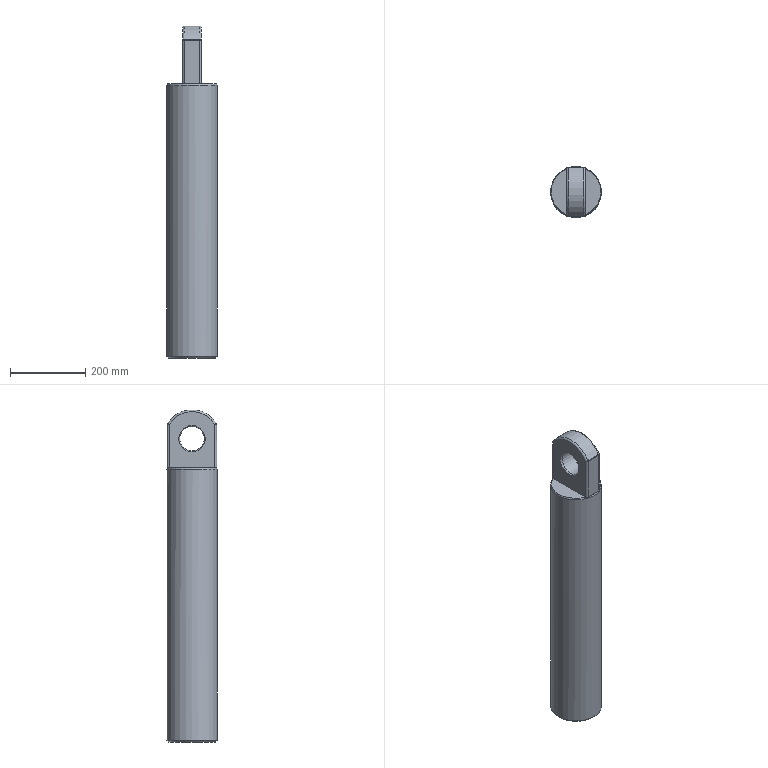Part | NX | features 平衡千斤顶活塞 2 | 1 solid | 32 faces | box 135 x 135 x 882.27 mm | volume 11180627 mm3 | plane 13 | cylinder 9 | cone 4 | sphere 4 | torus 2 | commonest cylinder face diameters 10 x6 65 x1 135 x1 153.5 x1
STEP:
#1=CARTESIAN_POINT('',(-24.997,60.688,727.9));
#2=VERTEX_POINT('',#1);
#3=CARTESIAN_POINT('',(-24.997,-60.688,727.9));
#4=VERTEX_POINT('',#3);
#5=CARTESIAN_POINT('',(0.,0.,727.9));
#6=DIRECTION('',(0.,0.,1.));
#7=DIRECTION('',(1.,0.,0.));
#8=AXIS2_PLACEMENT_3D('',#5,#6,#7);
#9=CIRCLE('',#8,65.635);
#10=EDGE_CURVE('',#2,#4,#9,.T.);
#11=ORIENTED_EDGE('',*,*,#10,.T.);
#12=CARTESIAN_POINT('',(-25.,-60.524,727.9));
#13=VERTEX_POINT('',#12);
#14=CARTESIAN_POINT('',(-20.,-60.524,727.9));
#15=DIRECTION('',(0.,0.,1.));
#16=DIRECTION('',(1.,0.,0.));
#17=AXIS2_PLACEMENT_3D('',#14,#15,#16);
#18=CIRCLE('',#17,5.);
#19=EDGE_CURVE('',#4,#13,#18,.F.);
#20=ORIENTED_EDGE('',*,*,#19,.T.);
#21=CARTESIAN_POINT('',(-25.,60.524,727.9));
#22=VERTEX_POINT('',#21);
#23=CARTESIAN_POINT('',(-25.,65.524,727.9));
#24=DIRECTION('',(0.,1.,0.));
#25=VECTOR('',#24,1000.);
#26=LINE('',#23,#25);
#27=EDGE_CURVE('',#13,#22,#26,.T.);
#28=ORIENTED_EDGE('',*,*,#27,.T.);
#29=CARTESIAN_POINT('',(-20.,60.524,727.9));
#30=DIRECTION('',(0.,0.,1.));
#31=DIRECTION('',(1.,0.,0.));
#32=AXIS2_PLACEMENT_3D('',#29,#30,#31);
#33=CIRCLE('',#32,5.);
#34=EDGE_CURVE('',#22,#2,#33,.F.);
#35=ORIENTED_EDGE('',*,*,#34,.T.);
#36=EDGE_LOOP('',(#11,#20,#28,#35));
#37=FACE_BOUND('',#36,.T.);
#38=CARTESIAN_POINT('',(0.,0.,727.9));
#39=DIRECTION('',(0.,0.,1.));
#40=DIRECTION('',(1.,0.,0.));
#41=AXIS2_PLACEMENT_3D('',#38,#39,#40);
#42=PLANE('',#41);
#43=ADVANCED_FACE('',(#37),#42,.T.);
#44=CARTESIAN_POINT('',(3.807,65.524,727.9));
#45=VERTEX_POINT('',#44);
#46=CARTESIAN_POINT('',(-3.807,65.524,727.9));
#47=VERTEX_POINT('',#46);
#48=CARTESIAN_POINT('',(25.,65.524,727.9));
#49=DIRECTION('',(-1.,0.,0.));
#50=VECTOR('',#49,1000.);
#51=LINE('',#48,#50);
#52=EDGE_CURVE('',#45,#47,#51,.T.);
#53=ORIENTED_EDGE('',*,*,#52,.F.);
#54=CARTESIAN_POINT('',(0.,0.,727.9));
#55=DIRECTION('',(0.,0.,1.));
#56=DIRECTION('',(1.,0.,0.));
#57=AXIS2_PLACEMENT_3D('',#54,#55,#56);
#58=CIRCLE('',#57,65.635);
#59=EDGE_CURVE('',#45,#47,#58,.T.);
#60=ORIENTED_EDGE('',*,*,#59,.T.);
#61=EDGE_LOOP('',(#53,#60));
#62=FACE_BOUND('',#61,.T.);
#63=CARTESIAN_POINT('',(0.,0.,727.9));
#64=DIRECTION('',(0.,0.,1.));
#65=DIRECTION('',(1.,0.,0.));
#66=AXIS2_PLACEMENT_3D('',#63,#64,#65);
#67=PLANE('',#66);
#68=ADVANCED_FACE('',(#62),#67,.T.);
#69=CARTESIAN_POINT('',(-3.816,-65.524,727.9));
#70=VERTEX_POINT('',#69);
#71=CARTESIAN_POINT('',(3.816,-65.524,727.9));
#72=VERTEX_POINT('',#71);
#73=CARTESIAN_POINT('',(0.,0.,727.9));
#74=DIRECTION('',(0.,0.,1.));
#75=DIRECTION('',(1.,0.,0.));
#76=AXIS2_PLACEMENT_3D('',#73,#74,#75);
#77=CIRCLE('',#76,65.635);
#78=EDGE_CURVE('',#70,#72,#77,.T.);
#79=ORIENTED_EDGE('',*,*,#78,.T.);
#80=CARTESIAN_POINT('',(25.,-65.524,727.9));
#81=DIRECTION('',(-1.,0.,0.));
#82=VECTOR('',#81,1000.);
#83=LINE('',#80,#82);
#84=EDGE_CURVE('',#72,#70,#83,.T.);
#85=ORIENTED_EDGE('',*,*,#84,.T.);
#86=EDGE_LOOP('',(#79,#85));
#87=FACE_BOUND('',#86,.T.);
#88=CARTESIAN_POINT('',(0.,0.,727.9));
#89=DIRECTION('',(0.,0.,1.));
#90=DIRECTION('',(1.,0.,0.));
#91=AXIS2_PLACEMENT_3D('',#88,#89,#90);
#92=PLANE('',#91);
#93=ADVANCED_FACE('',(#87),#92,.T.);
#94=CARTESIAN_POINT('',(67.5,0.,723.9));
#95=VERTEX_POINT('',#94);
#96=CARTESIAN_POINT('',(0.,0.,723.9));
#97=DIRECTION('',(0.,0.,1.));
#98=DIRECTION('',(1.,0.,0.));
#99=AXIS2_PLACEMENT_3D('',#96,#97,#98);
#100=CIRCLE('',#99,67.5);
#101=EDGE_CURVE('',#95,#95,#100,.F.);
#102=ORIENTED_EDGE('',*,*,#101,.T.);
#103=EDGE_LOOP('',(#102));
#104=FACE_BOUND('',#103,.T.);
#105=CARTESIAN_POINT('',(67.5,0.,5.));
#106=VERTEX_POINT('',#105);
#107=CARTESIAN_POINT('',(0.,0.,5.));
#108=DIRECTION('',(0.,0.,1.));
#109=DIRECTION('',(1.,0.,0.));
#110=AXIS2_PLACEMENT_3D('',#107,#108,#109);
#111=CIRCLE('',#110,67.5);
#112=EDGE_CURVE('',#106,#106,#111,.T.);
#113=ORIENTED_EDGE('',*,*,#112,.T.);
#114=EDGE_LOOP('',(#113));
#115=FACE_BOUND('',#114,.T.);
#116=CARTESIAN_POINT('',(0.,0.,727.9));
#117=DIRECTION('',(0.,0.,-1.));
#118=DIRECTION('',(-1.,0.,0.));
#119=AXIS2_PLACEMENT_3D('',#116,#117,#118);
#120=CYLINDRICAL_SURFACE('',#119,67.5);
#121=ADVANCED_FACE('',(#104,#115),#120,.T.);
#122=CARTESIAN_POINT('',(25.,-60.524,727.9));
#123=VERTEX_POINT('',#122);
#124=CARTESIAN_POINT('',(25.,60.524,727.9));
#125=VERTEX_POINT('',#124);
#126=CARTESIAN_POINT('',(25.,65.524,727.9));
#127=DIRECTION('',(0.,1.,0.));
#128=VECTOR('',#127,1000.);
#129=LINE('',#126,#128);
#130=EDGE_CURVE('',#123,#125,#129,.T.);
#131=ORIENTED_EDGE('',*,*,#130,.F.);
#132=CARTESIAN_POINT('',(24.997,-60.688,727.9));
#133=VERTEX_POINT('',#132);
#134=CARTESIAN_POINT('',(20.,-60.524,727.9));
#135=DIRECTION('',(0.,0.,1.));
#136=DIRECTION('',(1.,0.,0.));
#137=AXIS2_PLACEMENT_3D('',#134,#135,#136);
#138=CIRCLE('',#137,5.);
#139=EDGE_CURVE('',#123,#133,#138,.F.);
#140=ORIENTED_EDGE('',*,*,#139,.T.);
#141=CARTESIAN_POINT('',(24.997,60.688,727.9));
#142=VERTEX_POINT('',#141);
#143=CARTESIAN_POINT('',(0.,0.,727.9));
#144=DIRECTION('',(0.,0.,1.));
#145=DIRECTION('',(1.,0.,0.));
#146=AXIS2_PLACEMENT_3D('',#143,#144,#145);
#147=CIRCLE('',#146,65.635);
#148=EDGE_CURVE('',#133,#142,#147,.T.);
#149=ORIENTED_EDGE('',*,*,#148,.T.);
#150=CARTESIAN_POINT('',(20.,60.524,727.9));
#151=DIRECTION('',(0.,0.,1.));
#152=DIRECTION('',(1.,0.,0.));
#153=AXIS2_PLACEMENT_3D('',#150,#151,#152);
#154=CIRCLE('',#153,5.);
#155=EDGE_CURVE('',#142,#125,#154,.F.);
#156=ORIENTED_EDGE('',*,*,#155,.T.);
#157=EDGE_LOOP('',(#131,#140,#149,#156));
#158=FACE_BOUND('',#157,.T.);
#159=CARTESIAN_POINT('',(0.,0.,727.9));
#160=DIRECTION('',(0.,0.,1.));
#161=DIRECTION('',(1.,0.,0.));
#162=AXIS2_PLACEMENT_3D('',#159,#160,#161);
#163=PLANE('',#162);
#164=ADVANCED_FACE('',(#158),#163,.T.);
#165=CARTESIAN_POINT('',(62.5,0.,0.));
#166=VERTEX_POINT('',#165);
#167=CARTESIAN_POINT('',(0.,0.,0.));
#168=DIRECTION('',(0.,0.,1.));
#169=DIRECTION('',(1.,0.,0.));
#170=AXIS2_PLACEMENT_3D('',#167,#168,#169);
#171=CIRCLE('',#170,62.5);
#172=EDGE_CURVE('',#166,#166,#171,.F.);
#173=ORIENTED_EDGE('',*,*,#172,.T.);
#174=EDGE_LOOP('',(#173));
#175=FACE_BOUND('',#174,.T.);
#176=CARTESIAN_POINT('',(0.,0.,0.));
#177=DIRECTION('',(0.,0.,1.));
#178=DIRECTION('',(1.,0.,0.));
#179=AXIS2_PLACEMENT_3D('',#176,#177,#178);
#180=PLANE('',#179);
#181=ADVANCED_FACE('',(#175),#180,.F.);
#182=ORIENTED_EDGE('',*,*,#172,.F.);
#183=EDGE_LOOP('',(#182));
#184=FACE_BOUND('',#183,.T.);
#185=ORIENTED_EDGE('',*,*,#112,.F.);
#186=EDGE_LOOP('',(#185));
#187=FACE_BOUND('',#186,.T.);
#188=CARTESIAN_POINT('',(0.,0.,5.));
#189=DIRECTION('',(0.,0.,1.));
#190=DIRECTION('',(1.,0.,0.));
#191=AXIS2_PLACEMENT_3D('',#188,#189,#190);
#192=CONICAL_SURFACE('',#191,67.5,0.7854);
#193=ADVANCED_FACE('',(#184,#187),#192,.T.);
#194=ORIENTED_EDGE('',*,*,#101,.F.);
#195=EDGE_LOOP('',(#194));
#196=FACE_BOUND('',#195,.T.);
#197=CARTESIAN_POINT('',(0.,0.,727.9));
#198=DIRECTION('',(0.,0.,1.));
#199=DIRECTION('',(1.,0.,0.));
#200=AXIS2_PLACEMENT_3D('',#197,#198,#199);
#201=CIRCLE('',#200,65.635);
#202=EDGE_CURVE('',#142,#45,#201,.T.);
#203=ORIENTED_EDGE('',*,*,#202,.F.);
#204=ORIENTED_EDGE('',*,*,#148,.F.);
#205=CARTESIAN_POINT('',(0.,0.,727.9));
#206=DIRECTION('',(0.,0.,1.));
#207=DIRECTION('',(1.,0.,0.));
#208=AXIS2_PLACEMENT_3D('',#205,#206,#207);
#209=CIRCLE('',#208,65.635);
#210=EDGE_CURVE('',#72,#133,#209,.T.);
#211=ORIENTED_EDGE('',*,*,#210,.F.);
#212=ORIENTED_EDGE('',*,*,#78,.F.);
#213=CARTESIAN_POINT('',(0.,0.,727.9));
#214=DIRECTION('',(0.,0.,1.));
#215=DIRECTION('',(1.,0.,0.));
#216=AXIS2_PLACEMENT_3D('',#213,#214,#215);
#217=CIRCLE('',#216,65.635);
#218=EDGE_CURVE('',#4,#70,#217,.T.);
#219=ORIENTED_EDGE('',*,*,#218,.F.);
#220=ORIENTED_EDGE('',*,*,#10,.F.);
#221=CARTESIAN_POINT('',(0.,0.,727.9));
#222=DIRECTION('',(0.,0.,1.));
#223=DIRECTION('',(1.,0.,0.));
#224=AXIS2_PLACEMENT_3D('',#221,#222,#223);
#225=CIRCLE('',#224,65.635);
#226=EDGE_CURVE('',#47,#2,#225,.T.);
#227=ORIENTED_EDGE('',*,*,#226,.F.);
#228=ORIENTED_EDGE('',*,*,#59,.F.);
#229=EDGE_LOOP('',(#203,#204,#211,#212,#219,#220,#227,#228));
#230=FACE_BOUND('',#229,.T.);
#231=CARTESIAN_POINT('',(0.,0.,727.9));
#232=DIRECTION('',(0.,0.,-1.));
#233=DIRECTION('',(-1.,0.,0.));
#234=AXIS2_PLACEMENT_3D('',#231,#232,#233);
#235=CONICAL_SURFACE('',#234,65.635,0.4363);
#236=ADVANCED_FACE('',(#196,#230),#235,.T.);
#237=CARTESIAN_POINT('',(20.,65.524,727.9));
#238=VERTEX_POINT('',#237);
#239=CARTESIAN_POINT('',(25.,65.524,727.9));
#240=DIRECTION('',(-1.,0.,0.));
#241=VECTOR('',#240,1000.);
#242=LINE('',#239,#241);
#243=EDGE_CURVE('',#238,#45,#242,.T.);
#244=ORIENTED_EDGE('',*,*,#243,.F.);
#245=CARTESIAN_POINT('',(20.,60.524,727.9));
#246=DIRECTION('',(0.,0.,1.));
#247=DIRECTION('',(1.,0.,0.));
#248=AXIS2_PLACEMENT_3D('',#245,#246,#247);
#249=CIRCLE('',#248,5.);
#250=EDGE_CURVE('',#238,#142,#249,.F.);
#251=ORIENTED_EDGE('',*,*,#250,.T.);
#252=ORIENTED_EDGE('',*,*,#202,.T.);
#253=EDGE_LOOP('',(#244,#251,#252));
#254=FACE_BOUND('',#253,.T.);
#255=CARTESIAN_POINT('',(25.,65.524,727.9));
#256=DIRECTION('',(0.,0.,1.));
#257=DIRECTION('',(1.,0.,0.));
#258=AXIS2_PLACEMENT_3D('',#255,#256,#257);
#259=PLANE('',#258);
#260=ADVANCED_FACE('',(#254),#259,.F.);
#261=ORIENTED_EDGE('',*,*,#226,.T.);
#262=CARTESIAN_POINT('',(-20.,65.524,727.9));
#263=VERTEX_POINT('',#262);
#264=CARTESIAN_POINT('',(-20.,60.524,727.9));
#265=DIRECTION('',(0.,0.,1.));
#266=DIRECTION('',(1.,0.,0.));
#267=AXIS2_PLACEMENT_3D('',#264,#265,#266);
#268=CIRCLE('',#267,5.);
#269=EDGE_CURVE('',#2,#263,#268,.F.);
#270=ORIENTED_EDGE('',*,*,#269,.T.);
#271=CARTESIAN_POINT('',(25.,65.524,727.9));
#272=DIRECTION('',(-1.,0.,0.));
#273=VECTOR('',#272,1000.);
#274=LINE('',#271,#273);
#275=EDGE_CURVE('',#47,#263,#274,.T.);
#276=ORIENTED_EDGE('',*,*,#275,.F.);
#277=EDGE_LOOP('',(#261,#270,#276));
#278=FACE_BOUND('',#277,.T.);
#279=CARTESIAN_POINT('',(25.,65.524,727.9));
#280=DIRECTION('',(0.,0.,1.));
#281=DIRECTION('',(1.,0.,0.));
#282=AXIS2_PLACEMENT_3D('',#279,#280,#281);
#283=PLANE('',#282);
#284=ADVANCED_FACE('',(#278),#283,.F.);
#285=CARTESIAN_POINT('',(-20.,-65.524,727.9));
#286=VERTEX_POINT('',#285);
#287=CARTESIAN_POINT('',(25.,-65.524,727.9));
#288=DIRECTION('',(-1.,0.,0.));
#289=VECTOR('',#288,1000.);
#290=LINE('',#287,#289);
#291=EDGE_CURVE('',#70,#286,#290,.T.);
#292=ORIENTED_EDGE('',*,*,#291,.T.);
#293=CARTESIAN_POINT('',(-20.,-60.524,727.9));
#294=DIRECTION('',(0.,0.,1.));
#295=DIRECTION('',(1.,0.,0.));
#296=AXIS2_PLACEMENT_3D('',#293,#294,#295);
#297=CIRCLE('',#296,5.);
#298=EDGE_CURVE('',#286,#4,#297,.F.);
#299=ORIENTED_EDGE('',*,*,#298,.T.);
#300=ORIENTED_EDGE('',*,*,#218,.T.);
#301=EDGE_LOOP('',(#292,#299,#300));
#302=FACE_BOUND('',#301,.T.);
#303=CARTESIAN_POINT('',(25.,65.524,727.9));
#304=DIRECTION('',(0.,0.,1.));
#305=DIRECTION('',(1.,0.,0.));
#306=AXIS2_PLACEMENT_3D('',#303,#304,#305);
#307=PLANE('',#306);
#308=ADVANCED_FACE('',(#302),#307,.F.);
#309=ORIENTED_EDGE('',*,*,#210,.T.);
#310=CARTESIAN_POINT('',(20.,-65.524,727.9));
#311=VERTEX_POINT('',#310);
#312=CARTESIAN_POINT('',(20.,-60.524,727.9));
#313=DIRECTION('',(0.,0.,1.));
#314=DIRECTION('',(1.,0.,0.));
#315=AXIS2_PLACEMENT_3D('',#312,#313,#314);
#316=CIRCLE('',#315,5.);
#317=EDGE_CURVE('',#133,#311,#316,.F.);
#318=ORIENTED_EDGE('',*,*,#317,.T.);
#319=CARTESIAN_POINT('',(25.,-65.524,727.9));
#320=DIRECTION('',(-1.,0.,0.));
#321=VECTOR('',#320,1000.);
#322=LINE('',#319,#321);
#323=EDGE_CURVE('',#311,#72,#322,.T.);
#324=ORIENTED_EDGE('',*,*,#323,.T.);
#325=EDGE_LOOP('',(#309,#318,#324));
#326=FACE_BOUND('',#325,.T.);
#327=CARTESIAN_POINT('',(25.,65.524,727.9));
#328=DIRECTION('',(0.,0.,1.));
#329=DIRECTION('',(1.,0.,0.));
#330=AXIS2_PLACEMENT_3D('',#327,#328,#329);
#331=PLANE('',#330);
#332=ADVANCED_FACE('',(#326),#331,.F.);
#333=CARTESIAN_POINT('',(25.,0.0002601,768.02));
#334=VERTEX_POINT('',#333);
#335=CARTESIAN_POINT('',(25.,0.0002601,805.52));
#336=DIRECTION('',(1.,0.,0.));
#337=DIRECTION('',(0.,0.,-1.));
#338=AXIS2_PLACEMENT_3D('',#335,#336,#337);
#339=CIRCLE('',#338,37.5);
#340=EDGE_CURVE('',#334,#334,#339,.F.);
#341=ORIENTED_EDGE('',*,*,#340,.T.);
#342=EDGE_LOOP('',(#341));
#343=FACE_BOUND('',#342,.T.);
#344=CARTESIAN_POINT('',(25.,60.524,844.055));
#345=VERTEX_POINT('',#344);
#346=CARTESIAN_POINT('',(25.,-60.524,844.055));
#347=VERTEX_POINT('',#346);
#348=CARTESIAN_POINT('',(25.,0.0002601,805.52));
#349=DIRECTION('',(1.,0.,0.));
#350=DIRECTION('',(0.,0.,-1.));
#351=AXIS2_PLACEMENT_3D('',#348,#349,#350);
#352=CIRCLE('',#351,71.75);
#353=EDGE_CURVE('',#345,#347,#352,.T.);
#354=ORIENTED_EDGE('',*,*,#353,.T.);
#355=CARTESIAN_POINT('',(25.,-60.524,727.9));
#356=DIRECTION('',(0.,0.,-1.));
#357=VECTOR('',#356,1000.);
#358=LINE('',#355,#357);
#359=EDGE_CURVE('',#347,#123,#358,.T.);
#360=ORIENTED_EDGE('',*,*,#359,.T.);
#361=ORIENTED_EDGE('',*,*,#130,.T.);
#362=CARTESIAN_POINT('',(25.,60.524,845.485));
#363=DIRECTION('',(0.,0.,1.));
#364=VECTOR('',#363,1000.);
#365=LINE('',#362,#364);
#366=EDGE_CURVE('',#125,#345,#365,.T.);
#367=ORIENTED_EDGE('',*,*,#366,.T.);
#368=EDGE_LOOP('',(#354,#360,#361,#367));
#369=FACE_BOUND('',#368,.T.);
#370=CARTESIAN_POINT('',(25.,0.0002601,805.52));
#371=DIRECTION('',(1.,0.,0.));
#372=DIRECTION('',(0.,0.,-1.));
#373=AXIS2_PLACEMENT_3D('',#370,#371,#372);
#374=PLANE('',#373);
#375=ADVANCED_FACE('',(#343,#369),#374,.T.);
#376=CARTESIAN_POINT('',(-25.,0.0002601,770.688));
#377=VERTEX_POINT('',#376);
#378=CARTESIAN_POINT('',(-25.,0.0002601,805.52));
#379=DIRECTION('',(1.,0.,0.));
#380=DIRECTION('',(0.,0.,-1.));
#381=AXIS2_PLACEMENT_3D('',#378,#379,#380);
#382=CIRCLE('',#381,34.832);
#383=EDGE_CURVE('',#377,#377,#382,.T.);
#384=ORIENTED_EDGE('',*,*,#383,.T.);
#385=EDGE_LOOP('',(#384));
#386=FACE_BOUND('',#385,.T.);
#387=ORIENTED_EDGE('',*,*,#27,.F.);
#388=CARTESIAN_POINT('',(-25.,-60.524,844.055));
#389=VERTEX_POINT('',#388);
#390=CARTESIAN_POINT('',(-25.,-60.524,805.52));
#391=DIRECTION('',(0.,0.,-1.));
#392=VECTOR('',#391,1000.);
#393=LINE('',#390,#392);
#394=EDGE_CURVE('',#13,#389,#393,.F.);
#395=ORIENTED_EDGE('',*,*,#394,.T.);
#396=CARTESIAN_POINT('',(-25.,60.524,844.055));
#397=VERTEX_POINT('',#396);
#398=CARTESIAN_POINT('',(-25.,0.0002601,805.52));
#399=DIRECTION('',(1.,0.,0.));
#400=DIRECTION('',(0.,0.,-1.));
#401=AXIS2_PLACEMENT_3D('',#398,#399,#400);
#402=CIRCLE('',#401,71.75);
#403=EDGE_CURVE('',#389,#397,#402,.F.);
#404=ORIENTED_EDGE('',*,*,#403,.T.);
#405=CARTESIAN_POINT('',(-25.,60.524,805.52));
#406=DIRECTION('',(0.,0.,1.));
#407=VECTOR('',#406,1000.);
#408=LINE('',#405,#407);
#409=EDGE_CURVE('',#397,#22,#408,.F.);
#410=ORIENTED_EDGE('',*,*,#409,.T.);
#411=EDGE_LOOP('',(#387,#395,#404,#410));
#412=FACE_BOUND('',#411,.T.);
#413=CARTESIAN_POINT('',(-25.,0.0002601,805.52));
#414=DIRECTION('',(1.,0.,0.));
#415=DIRECTION('',(0.,0.,-1.));
#416=AXIS2_PLACEMENT_3D('',#413,#414,#415);
#417=PLANE('',#416);
#418=ADVANCED_FACE('',(#386,#412),#417,.F.);
#419=CARTESIAN_POINT('',(-20.,65.524,844.055));
#420=VERTEX_POINT('',#419);
#421=CARTESIAN_POINT('',(20.,65.524,844.055));
#422=VERTEX_POINT('',#421);
#423=CARTESIAN_POINT('',(25.,65.524,844.055));
#424=DIRECTION('',(-1.,0.,0.));
#425=VECTOR('',#424,1000.);
#426=LINE('',#423,#425);
#427=EDGE_CURVE('',#420,#422,#426,.F.);
#428=ORIENTED_EDGE('',*,*,#427,.T.);
#429=CARTESIAN_POINT('',(20.,65.524,727.9));
#430=DIRECTION('',(0.,0.,1.));
#431=VECTOR('',#430,1000.);
#432=LINE('',#429,#431);
#433=EDGE_CURVE('',#422,#238,#432,.F.);
#434=ORIENTED_EDGE('',*,*,#433,.T.);
#435=ORIENTED_EDGE('',*,*,#243,.T.);
#436=ORIENTED_EDGE('',*,*,#52,.T.);
#437=ORIENTED_EDGE('',*,*,#275,.T.);
#438=CARTESIAN_POINT('',(-20.,65.524,727.9));
#439=DIRECTION('',(0.,0.,1.));
#440=VECTOR('',#439,1000.);
#441=LINE('',#438,#440);
#442=EDGE_CURVE('',#263,#420,#441,.T.);
#443=ORIENTED_EDGE('',*,*,#442,.T.);
#444=EDGE_LOOP('',(#428,#434,#435,#436,#437,#443));
#445=FACE_BOUND('',#444,.T.);
#446=CARTESIAN_POINT('',(25.,65.524,727.9));
#447=DIRECTION('',(0.,-1.,0.));
#448=DIRECTION('',(0.,0.,-1.));
#449=AXIS2_PLACEMENT_3D('',#446,#447,#448);
#450=PLANE('',#449);
#451=ADVANCED_FACE('',(#445),#450,.F.);
#452=CARTESIAN_POINT('',(20.,-64.741,846.74));
#453=VERTEX_POINT('',#452);
#454=CARTESIAN_POINT('',(20.,64.742,846.74));
#455=VERTEX_POINT('',#454);
#456=CARTESIAN_POINT('',(20.,0.0002601,805.52));
#457=DIRECTION('',(1.,0.,0.));
#458=DIRECTION('',(0.,0.,-1.));
#459=AXIS2_PLACEMENT_3D('',#456,#457,#458);
#460=CIRCLE('',#459,76.75);
#461=EDGE_CURVE('',#453,#455,#460,.F.);
#462=ORIENTED_EDGE('',*,*,#461,.T.);
#463=CARTESIAN_POINT('',(-20.,64.742,846.74));
#464=VERTEX_POINT('',#463);
#465=CARTESIAN_POINT('',(25.,64.742,846.74));
#466=DIRECTION('',(-1.,0.,0.));
#467=VECTOR('',#466,1000.);
#468=LINE('',#465,#467);
#469=EDGE_CURVE('',#455,#464,#468,.T.);
#470=ORIENTED_EDGE('',*,*,#469,.T.);
#471=CARTESIAN_POINT('',(-20.,-64.741,846.74));
#472=VERTEX_POINT('',#471);
#473=CARTESIAN_POINT('',(-20.,0.0002601,805.52));
#474=DIRECTION('',(1.,0.,0.));
#475=DIRECTION('',(0.,0.,-1.));
#476=AXIS2_PLACEMENT_3D('',#473,#474,#475);
#477=CIRCLE('',#476,76.75);
#478=EDGE_CURVE('',#464,#472,#477,.T.);
#479=ORIENTED_EDGE('',*,*,#478,.T.);
#480=CARTESIAN_POINT('',(25.,-64.741,846.74));
#481=DIRECTION('',(-1.,0.,0.));
#482=VECTOR('',#481,1000.);
#483=LINE('',#480,#482);
#484=EDGE_CURVE('',#472,#453,#483,.F.);
#485=ORIENTED_EDGE('',*,*,#484,.T.);
#486=EDGE_LOOP('',(#462,#470,#479,#485));
#487=FACE_BOUND('',#486,.T.);
#488=CARTESIAN_POINT('',(25.,0.0002601,805.52));
#489=DIRECTION('',(-1.,0.,0.));
#490=DIRECTION('',(0.,0.,1.));
#491=AXIS2_PLACEMENT_3D('',#488,#489,#490);
#492=CYLINDRICAL_SURFACE('',#491,76.75);
#493=ADVANCED_FACE('',(#487),#492,.T.);
#494=ORIENTED_EDGE('',*,*,#323,.F.);
#495=CARTESIAN_POINT('',(20.,-65.524,844.055));
#496=VERTEX_POINT('',#495);
#497=CARTESIAN_POINT('',(20.,-65.524,845.485));
#498=DIRECTION('',(0.,0.,-1.));
#499=VECTOR('',#498,1000.);
#500=LINE('',#497,#499);
#501=EDGE_CURVE('',#311,#496,#500,.F.);
#502=ORIENTED_EDGE('',*,*,#501,.T.);
#503=CARTESIAN_POINT('',(-20.,-65.524,844.055));
#504=VERTEX_POINT('',#503);
#505=CARTESIAN_POINT('',(25.,-65.524,844.055));
#506=DIRECTION('',(-1.,0.,0.));
#507=VECTOR('',#506,1000.);
#508=LINE('',#505,#507);
#509=EDGE_CURVE('',#496,#504,#508,.T.);
#510=ORIENTED_EDGE('',*,*,#509,.T.);
#511=CARTESIAN_POINT('',(-20.,-65.524,727.9));
#512=DIRECTION('',(0.,0.,-1.));
#513=VECTOR('',#512,1000.);
#514=LINE('',#511,#513);
#515=EDGE_CURVE('',#504,#286,#514,.T.);
#516=ORIENTED_EDGE('',*,*,#515,.T.);
#517=ORIENTED_EDGE('',*,*,#291,.F.);
#518=ORIENTED_EDGE('',*,*,#84,.F.);
#519=EDGE_LOOP('',(#494,#502,#510,#516,#517,#518));
#520=FACE_BOUND('',#519,.T.);
#521=CARTESIAN_POINT('',(25.,-65.524,727.9));
#522=DIRECTION('',(0.,1.,0.));
#523=DIRECTION('',(0.,0.,1.));
#524=AXIS2_PLACEMENT_3D('',#521,#522,#523);
#525=PLANE('',#524);
#526=ADVANCED_FACE('',(#520),#525,.F.);
#527=CARTESIAN_POINT('',(22.668,0.0002601,773.02));
#528=VERTEX_POINT('',#527);
#529=CARTESIAN_POINT('',(22.668,0.0002601,805.52));
#530=DIRECTION('',(1.,0.,0.));
#531=DIRECTION('',(0.,0.,-1.));
#532=AXIS2_PLACEMENT_3D('',#529,#530,#531);
#533=CIRCLE('',#532,32.5);
#534=EDGE_CURVE('',#528,#528,#533,.T.);
#535=ORIENTED_EDGE('',*,*,#534,.T.);
#536=EDGE_LOOP('',(#535));
#537=FACE_BOUND('',#536,.T.);
#538=CARTESIAN_POINT('',(-20.,0.0002601,773.02));
#539=VERTEX_POINT('',#538);
#540=CARTESIAN_POINT('',(-20.,0.0002601,805.52));
#541=DIRECTION('',(1.,0.,0.));
#542=DIRECTION('',(0.,0.,-1.));
#543=AXIS2_PLACEMENT_3D('',#540,#541,#542);
#544=CIRCLE('',#543,32.5);
#545=EDGE_CURVE('',#539,#539,#544,.F.);
#546=ORIENTED_EDGE('',*,*,#545,.T.);
#547=EDGE_LOOP('',(#546));
#548=FACE_BOUND('',#547,.T.);
#549=CARTESIAN_POINT('',(25.,0.0002601,805.52));
#550=DIRECTION('',(-1.,0.,0.));
#551=DIRECTION('',(0.,0.,1.));
#552=AXIS2_PLACEMENT_3D('',#549,#550,#551);
#553=CYLINDRICAL_SURFACE('',#552,32.5);
#554=ADVANCED_FACE('',(#537,#548),#553,.F.);
#555=ORIENTED_EDGE('',*,*,#139,.F.);
#556=ORIENTED_EDGE('',*,*,#359,.F.);
#557=CARTESIAN_POINT('',(20.,-60.524,844.055));
#558=DIRECTION('',(0.,0.,1.));
#559=DIRECTION('',(1.,0.,0.));
#560=AXIS2_PLACEMENT_3D('',#557,#558,#559);
#561=CIRCLE('',#560,5.);
#562=EDGE_CURVE('',#496,#347,#561,.T.);
#563=ORIENTED_EDGE('',*,*,#562,.F.);
#564=ORIENTED_EDGE('',*,*,#501,.F.);
#565=ORIENTED_EDGE('',*,*,#317,.F.);
#566=EDGE_LOOP('',(#555,#556,#563,#564,#565));
#567=FACE_BOUND('',#566,.T.);
#568=CARTESIAN_POINT('',(20.,-60.524,805.52));
#569=DIRECTION('',(0.,0.,1.));
#570=DIRECTION('',(1.,0.,0.));
#571=AXIS2_PLACEMENT_3D('',#568,#569,#570);
#572=CYLINDRICAL_SURFACE('',#571,5.);
#573=ADVANCED_FACE('',(#567),#572,.T.);
#574=CARTESIAN_POINT('',(-20.,-60.524,844.055));
#575=DIRECTION('',(-1.,0.,0.));
#576=DIRECTION('',(0.,0.,1.));
#577=AXIS2_PLACEMENT_3D('',#574,#575,#576);
#578=CIRCLE('',#577,5.);
#579=EDGE_CURVE('',#504,#472,#578,.T.);
#580=ORIENTED_EDGE('',*,*,#579,.F.);
#581=ORIENTED_EDGE('',*,*,#509,.F.);
#582=CARTESIAN_POINT('',(20.,-60.524,844.055));
#583=DIRECTION('',(1.,0.,0.));
#584=DIRECTION('',(0.,0.,-1.));
#585=AXIS2_PLACEMENT_3D('',#582,#583,#584);
#586=CIRCLE('',#585,5.);
#587=EDGE_CURVE('',#453,#496,#586,.T.);
#588=ORIENTED_EDGE('',*,*,#587,.F.);
#589=ORIENTED_EDGE('',*,*,#484,.F.);
#590=EDGE_LOOP('',(#580,#581,#588,#589));
#591=FACE_BOUND('',#590,.T.);
#592=CARTESIAN_POINT('',(25.,-60.524,844.055));
#593=DIRECTION('',(-1.,0.,0.));
#594=DIRECTION('',(0.,0.,1.));
#595=AXIS2_PLACEMENT_3D('',#592,#593,#594);
#596=CYLINDRICAL_SURFACE('',#595,5.);
#597=ADVANCED_FACE('',(#591),#596,.T.);
#598=ORIENTED_EDGE('',*,*,#298,.F.);
#599=ORIENTED_EDGE('',*,*,#515,.F.);
#600=CARTESIAN_POINT('',(-20.,-60.524,844.055));
#601=DIRECTION('',(0.,0.,1.));
#602=DIRECTION('',(1.,0.,0.));
#603=AXIS2_PLACEMENT_3D('',#600,#601,#602);
#604=CIRCLE('',#603,5.);
#605=EDGE_CURVE('',#389,#504,#604,.T.);
#606=ORIENTED_EDGE('',*,*,#605,.F.);
#607=ORIENTED_EDGE('',*,*,#394,.F.);
#608=ORIENTED_EDGE('',*,*,#19,.F.);
#609=EDGE_LOOP('',(#598,#599,#606,#607,#608));
#610=FACE_BOUND('',#609,.T.);
#611=CARTESIAN_POINT('',(-20.,-60.524,727.9));
#612=DIRECTION('',(0.,0.,-1.));
#613=DIRECTION('',(-1.,0.,0.));
#614=AXIS2_PLACEMENT_3D('',#611,#612,#613);
#615=CYLINDRICAL_SURFACE('',#614,5.);
#616=ADVANCED_FACE('',(#610),#615,.T.);
#617=ORIENTED_EDGE('',*,*,#587,.T.);
#618=ORIENTED_EDGE('',*,*,#562,.T.);
#619=CARTESIAN_POINT('',(20.,-60.524,844.055));
#620=DIRECTION('',(0.,-0.5371,-0.8435));
#621=DIRECTION('',(0.,0.8435,-0.5371));
#622=AXIS2_PLACEMENT_3D('',#619,#620,#621);
#623=CIRCLE('',#622,5.);
#624=EDGE_CURVE('',#453,#347,#623,.F.);
#625=ORIENTED_EDGE('',*,*,#624,.F.);
#626=EDGE_LOOP('',(#617,#618,#625));
#627=FACE_BOUND('',#626,.T.);
#628=CARTESIAN_POINT('',(20.,-60.524,844.055));
#629=DIRECTION('',(0.,0.,1.));
#630=DIRECTION('',(1.,0.,0.));
#631=AXIS2_PLACEMENT_3D('',#628,#629,#630);
#632=SPHERICAL_SURFACE('',#631,5.);
#633=ADVANCED_FACE('',(#627),#632,.T.);
#634=ORIENTED_EDGE('',*,*,#605,.T.);
#635=ORIENTED_EDGE('',*,*,#579,.T.);
#636=CARTESIAN_POINT('',(-20.,-60.524,844.055));
#637=DIRECTION('',(0.,-0.5371,-0.8435));
#638=DIRECTION('',(0.,0.8435,-0.5371));
#639=AXIS2_PLACEMENT_3D('',#636,#637,#638);
#640=CIRCLE('',#639,5.);
#641=EDGE_CURVE('',#389,#472,#640,.F.);
#642=ORIENTED_EDGE('',*,*,#641,.F.);
#643=EDGE_LOOP('',(#634,#635,#642));
#644=FACE_BOUND('',#643,.T.);
#645=CARTESIAN_POINT('',(-20.,-60.524,844.055));
#646=DIRECTION('',(0.,0.,1.));
#647=DIRECTION('',(1.,0.,0.));
#648=AXIS2_PLACEMENT_3D('',#645,#646,#647);
#649=SPHERICAL_SURFACE('',#648,5.);
#650=ADVANCED_FACE('',(#644),#649,.T.);
#651=ORIENTED_EDGE('',*,*,#250,.F.);
#652=ORIENTED_EDGE('',*,*,#433,.F.);
#653=CARTESIAN_POINT('',(20.,60.524,844.055));
#654=DIRECTION('',(0.,0.,1.));
#655=DIRECTION('',(1.,0.,0.));
#656=AXIS2_PLACEMENT_3D('',#653,#654,#655);
#657=CIRCLE('',#656,5.);
#658=EDGE_CURVE('',#345,#422,#657,.T.);
#659=ORIENTED_EDGE('',*,*,#658,.F.);
#660=ORIENTED_EDGE('',*,*,#366,.F.);
#661=ORIENTED_EDGE('',*,*,#155,.F.);
#662=EDGE_LOOP('',(#651,#652,#659,#660,#661));
#663=FACE_BOUND('',#662,.T.);
#664=CARTESIAN_POINT('',(20.,60.524,805.52));
#665=DIRECTION('',(0.,0.,-1.));
#666=DIRECTION('',(0.,1.,0.));
#667=AXIS2_PLACEMENT_3D('',#664,#665,#666);
#668=CYLINDRICAL_SURFACE('',#667,5.);
#669=ADVANCED_FACE('',(#663),#668,.T.);
#670=ORIENTED_EDGE('',*,*,#624,.T.);
#671=ORIENTED_EDGE('',*,*,#353,.F.);
#672=CARTESIAN_POINT('',(20.,60.524,844.055));
#673=DIRECTION('',(0.,0.5371,-0.8435));
#674=DIRECTION('',(0.,0.8435,0.5371));
#675=AXIS2_PLACEMENT_3D('',#672,#673,#674);
#676=CIRCLE('',#675,5.);
#677=EDGE_CURVE('',#455,#345,#676,.T.);
#678=ORIENTED_EDGE('',*,*,#677,.F.);
#679=ORIENTED_EDGE('',*,*,#461,.F.);
#680=EDGE_LOOP('',(#670,#671,#678,#679));
#681=FACE_BOUND('',#680,.T.);
#682=CARTESIAN_POINT('',(20.,0.0002601,805.52));
#683=DIRECTION('',(1.,0.,0.));
#684=DIRECTION('',(0.,0.,-1.));
#685=AXIS2_PLACEMENT_3D('',#682,#683,#684);
#686=TOROIDAL_SURFACE('',#685,71.75,5.);
#687=ADVANCED_FACE('',(#681),#686,.T.);
#688=ORIENTED_EDGE('',*,*,#641,.T.);
#689=ORIENTED_EDGE('',*,*,#478,.F.);
#690=CARTESIAN_POINT('',(-20.,60.524,844.055));
#691=DIRECTION('',(0.,0.5371,-0.8435));
#692=DIRECTION('',(0.,0.8435,0.5371));
#693=AXIS2_PLACEMENT_3D('',#690,#691,#692);
#694=CIRCLE('',#693,5.);
#695=EDGE_CURVE('',#397,#464,#694,.T.);
#696=ORIENTED_EDGE('',*,*,#695,.F.);
#697=ORIENTED_EDGE('',*,*,#403,.F.);
#698=EDGE_LOOP('',(#688,#689,#696,#697));
#699=FACE_BOUND('',#698,.T.);
#700=CARTESIAN_POINT('',(-20.,0.0002601,805.52));
#701=DIRECTION('',(1.,0.,0.));
#702=DIRECTION('',(0.,0.,-1.));
#703=AXIS2_PLACEMENT_3D('',#700,#701,#702);
#704=TOROIDAL_SURFACE('',#703,71.75,5.);
#705=ADVANCED_FACE('',(#699),#704,.T.);
#706=ORIENTED_EDGE('',*,*,#34,.F.);
#707=ORIENTED_EDGE('',*,*,#409,.F.);
#708=CARTESIAN_POINT('',(-20.,60.524,844.055));
#709=DIRECTION('',(0.,0.,1.));
#710=DIRECTION('',(1.,0.,0.));
#711=AXIS2_PLACEMENT_3D('',#708,#709,#710);
#712=CIRCLE('',#711,5.);
#713=EDGE_CURVE('',#420,#397,#712,.T.);
#714=ORIENTED_EDGE('',*,*,#713,.F.);
#715=ORIENTED_EDGE('',*,*,#442,.F.);
#716=ORIENTED_EDGE('',*,*,#269,.F.);
#717=EDGE_LOOP('',(#706,#707,#714,#715,#716));
#718=FACE_BOUND('',#717,.T.);
#719=CARTESIAN_POINT('',(-20.,60.524,727.9));
#720=DIRECTION('',(0.,0.,1.));
#721=DIRECTION('',(0.,-1.,0.));
#722=AXIS2_PLACEMENT_3D('',#719,#720,#721);
#723=CYLINDRICAL_SURFACE('',#722,5.);
#724=ADVANCED_FACE('',(#718),#723,.T.);
#725=ORIENTED_EDGE('',*,*,#677,.T.);
#726=ORIENTED_EDGE('',*,*,#658,.T.);
#727=CARTESIAN_POINT('',(20.,60.524,844.055));
#728=DIRECTION('',(1.,0.,0.));
#729=DIRECTION('',(0.,0.,-1.));
#730=AXIS2_PLACEMENT_3D('',#727,#728,#729);
#731=CIRCLE('',#730,5.);
#732=EDGE_CURVE('',#455,#422,#731,.F.);
#733=ORIENTED_EDGE('',*,*,#732,.F.);
#734=EDGE_LOOP('',(#725,#726,#733));
#735=FACE_BOUND('',#734,.T.);
#736=CARTESIAN_POINT('',(20.,60.524,844.055));
#737=DIRECTION('',(0.,0.,1.));
#738=DIRECTION('',(1.,0.,0.));
#739=AXIS2_PLACEMENT_3D('',#736,#737,#738);
#740=SPHERICAL_SURFACE('',#739,5.);
#741=ADVANCED_FACE('',(#735),#740,.T.);
#742=ORIENTED_EDGE('',*,*,#713,.T.);
#743=ORIENTED_EDGE('',*,*,#695,.T.);
#744=CARTESIAN_POINT('',(-20.,60.524,844.055));
#745=DIRECTION('',(-1.,0.,0.));
#746=DIRECTION('',(0.,0.,1.));
#747=AXIS2_PLACEMENT_3D('',#744,#745,#746);
#748=CIRCLE('',#747,5.);
#749=EDGE_CURVE('',#420,#464,#748,.F.);
#750=ORIENTED_EDGE('',*,*,#749,.F.);
#751=EDGE_LOOP('',(#742,#743,#750));
#752=FACE_BOUND('',#751,.T.);
#753=CARTESIAN_POINT('',(-20.,60.524,844.055));
#754=DIRECTION('',(0.,0.,1.));
#755=DIRECTION('',(1.,0.,0.));
#756=AXIS2_PLACEMENT_3D('',#753,#754,#755);
#757=SPHERICAL_SURFACE('',#756,5.);
#758=ADVANCED_FACE('',(#752),#757,.T.);
#759=ORIENTED_EDGE('',*,*,#732,.T.);
#760=ORIENTED_EDGE('',*,*,#427,.F.);
#761=ORIENTED_EDGE('',*,*,#749,.T.);
#762=ORIENTED_EDGE('',*,*,#469,.F.);
#763=EDGE_LOOP('',(#759,#760,#761,#762));
#764=FACE_BOUND('',#763,.T.);
#765=CARTESIAN_POINT('',(25.,60.524,844.055));
#766=DIRECTION('',(-1.,0.,0.));
#767=DIRECTION('',(0.,0.,1.));
#768=AXIS2_PLACEMENT_3D('',#765,#766,#767);
#769=CYLINDRICAL_SURFACE('',#768,5.);
#770=ADVANCED_FACE('',(#764),#769,.T.);
#771=ORIENTED_EDGE('',*,*,#340,.F.);
#772=EDGE_LOOP('',(#771));
#773=FACE_BOUND('',#772,.T.);
#774=ORIENTED_EDGE('',*,*,#534,.F.);
#775=EDGE_LOOP('',(#774));
#776=FACE_BOUND('',#775,.T.);
#777=CARTESIAN_POINT('',(22.668,0.0002601,805.52));
#778=DIRECTION('',(1.,0.,0.));
#779=DIRECTION('',(0.,0.,-1.));
#780=AXIS2_PLACEMENT_3D('',#777,#778,#779);
#781=CONICAL_SURFACE('',#780,32.5,1.134);
#782=ADVANCED_FACE('',(#773,#776),#781,.F.);
#783=ORIENTED_EDGE('',*,*,#545,.F.);
#784=EDGE_LOOP('',(#783));
#785=FACE_BOUND('',#784,.T.);
#786=ORIENTED_EDGE('',*,*,#383,.F.);
#787=EDGE_LOOP('',(#786));
#788=FACE_BOUND('',#787,.T.);
#789=CARTESIAN_POINT('',(-25.,0.0002601,805.52));
#790=DIRECTION('',(-1.,0.,0.));
#791=DIRECTION('',(0.,0.,1.));
#792=AXIS2_PLACEMENT_3D('',#789,#790,#791);
#793=CONICAL_SURFACE('',#792,34.832,0.4363);
#794=ADVANCED_FACE('',(#785,#788),#793,.F.);
#795=CLOSED_SHELL('',(#43,#68,#93,#121,#164,#181,#193,#236,#260,#284,#308,#332,#375,#418,#451,#493,#526,#554,#573,#597,#616,#633,#650,#669,#687,#705,#724,#741,#758,#770,#782,#794));
#796=MANIFOLD_SOLID_BREP('',#795);
#797=(LENGTH_UNIT()NAMED_UNIT(*)SI_UNIT(.MILLI.,.METRE.));
#798=UNCERTAINTY_MEASURE_WITH_UNIT(LENGTH_MEASURE(0.00001),#797,'','');
#799=(NAMED_UNIT(*)PLANE_ANGLE_UNIT()SI_UNIT($,.RADIAN.));
#800=(NAMED_UNIT(*)SI_UNIT($,.STERADIAN.)SOLID_ANGLE_UNIT());
#801=(GEOMETRIC_REPRESENTATION_CONTEXT(3)GLOBAL_UNCERTAINTY_ASSIGNED_CONTEXT((#798))GLOBAL_UNIT_ASSIGNED_CONTEXT((#797,#799,#800))REPRESENTATION_CONTEXT('',''));
#802=ADVANCED_BREP_SHAPE_REPRESENTATION('',(#796),#801);